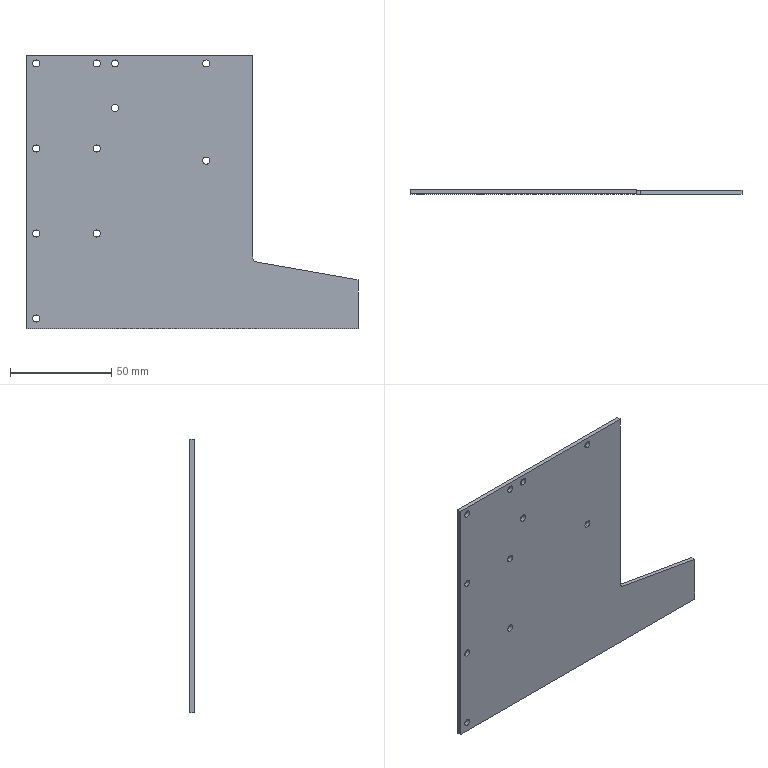Part | STEP file | Screw feeder-hopper side plate_default | 1 solid | 31 faces | box 164 x 2 x 135 mm | volume 33017 mm3 | cylinder 23 | plane 8 | commonest cylinder face diameters 3.5 x22 5 x1